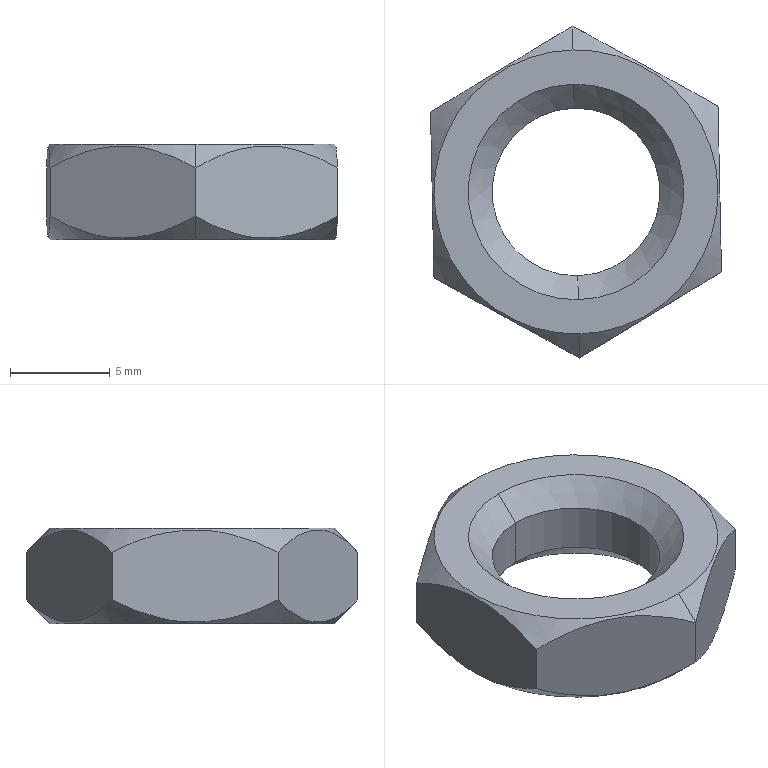Part | SolidWorks | features BaseBody 1 | 1 solid | 18 faces | box 14.572 x 16.624 x 4.802 mm | volume 539.911 mm3 | cone 8 | plane 8 | cylinder 2 | commonest cylinder face diameters 8.4 x2
STEP:
#1=CARTESIAN_POINT('',(341.861,193.205,-8.525));
#2=VERTEX_POINT('',#1);
#3=CARTESIAN_POINT('',(341.685,201.603,-8.525));
#4=VERTEX_POINT('',#3);
#5=CARTESIAN_POINT('',(341.773,197.404,-8.525));
#6=DIRECTION('',(-0.0001435,-0.000000521,1.));
#7=DIRECTION('',(0.02104,-0.9998,0.000002497));
#8=AXIS2_PLACEMENT_3D('',#5,#6,#7);
#9=CIRCLE('',#8,4.2);
#10=EDGE_CURVE('',#2,#4,#9,.T.);
#11=ORIENTED_EDGE('',*,*,#10,.T.);
#12=CARTESIAN_POINT('',(341.659,202.802,-9.725));
#13=VERTEX_POINT('',#12);
#14=CARTESIAN_POINT('',(341.672,202.203,-9.125));
#15=DIRECTION('',(-0.01477,0.707,-0.7071));
#16=VECTOR('',#15,1000.);
#17=LINE('',#14,#16);
#18=EDGE_CURVE('',#4,#13,#17,.T.);
#19=ORIENTED_EDGE('',*,*,#18,.T.);
#20=CARTESIAN_POINT('',(341.887,192.005,-9.725));
#21=VERTEX_POINT('',#20);
#22=CARTESIAN_POINT('',(341.773,197.404,-9.725));
#23=DIRECTION('',(-0.0001435,-0.000000521,1.));
#24=DIRECTION('',(-0.02104,0.9998,-0.000002497));
#25=AXIS2_PLACEMENT_3D('',#22,#23,#24);
#26=CIRCLE('',#25,5.4);
#27=EDGE_CURVE('',#21,#13,#26,.T.);
#28=ORIENTED_EDGE('',*,*,#27,.F.);
#29=CARTESIAN_POINT('',(341.874,192.605,-9.125));
#30=DIRECTION('',(0.01498,-0.7069,-0.7071));
#31=VECTOR('',#30,1000.);
#32=LINE('',#29,#31);
#33=EDGE_CURVE('',#2,#21,#32,.T.);
#34=ORIENTED_EDGE('',*,*,#33,.F.);
#35=EDGE_LOOP('',(#11,#19,#28,#34));
#36=FACE_OUTER_BOUND('',#35,.T.);
#37=CARTESIAN_POINT('',(341.773,197.404,-9.125));
#38=DIRECTION('',(0.0001435,0.000000521,-1.));
#39=DIRECTION('',(0.02104,-0.9998,0.000002497));
#40=AXIS2_PLACEMENT_3D('',#37,#38,#39);
#41=CONICAL_SURFACE('',#40,4.8,0.7854);
#42=ADVANCED_FACE('',(#36),#41,.F.);
#43=CARTESIAN_POINT('',(341.684,201.603,-6.125));
#44=VERTEX_POINT('',#43);
#45=CARTESIAN_POINT('',(341.861,193.205,-6.125));
#46=VERTEX_POINT('',#45);
#47=CARTESIAN_POINT('',(341.773,197.404,-6.125));
#48=DIRECTION('',(0.0001435,0.000000521,-1.));
#49=DIRECTION('',(0.02104,-0.9998,0.000002497));
#50=AXIS2_PLACEMENT_3D('',#47,#48,#49);
#51=CIRCLE('',#50,4.2);
#52=EDGE_CURVE('',#44,#46,#51,.T.);
#53=ORIENTED_EDGE('',*,*,#52,.F.);
#54=CARTESIAN_POINT('',(341.684,201.603,-3.125));
#55=DIRECTION('',(0.0001435,0.000000521,-1.));
#56=VECTOR('',#55,1000.);
#57=LINE('',#54,#56);
#58=EDGE_CURVE('',#44,#4,#57,.T.);
#59=ORIENTED_EDGE('',*,*,#58,.T.);
#60=ORIENTED_EDGE('',*,*,#10,.F.);
#61=CARTESIAN_POINT('',(341.86,193.205,-3.125));
#62=DIRECTION('',(0.0001435,0.000000521,-1.));
#63=VECTOR('',#62,1000.);
#64=LINE('',#61,#63);
#65=EDGE_CURVE('',#46,#2,#64,.T.);
#66=ORIENTED_EDGE('',*,*,#65,.F.);
#67=EDGE_LOOP('',(#53,#59,#60,#66));
#68=FACE_OUTER_BOUND('',#67,.T.);
#69=CARTESIAN_POINT('',(341.772,197.404,-3.125));
#70=DIRECTION('',(0.0001435,0.000000521,-1.));
#71=DIRECTION('',(0.02104,-0.9998,0.000002497));
#72=AXIS2_PLACEMENT_3D('',#69,#70,#71);
#73=CYLINDRICAL_SURFACE('',#72,4.2);
#74=ADVANCED_FACE('',(#68),#73,.F.);
#75=ORIENTED_EDGE('',*,*,#52,.T.);
#76=CARTESIAN_POINT('',(341.886,192.005,-4.925));
#77=VERTEX_POINT('',#76);
#78=CARTESIAN_POINT('',(341.873,192.605,-5.525));
#79=DIRECTION('',(0.01477,-0.707,0.7071));
#80=VECTOR('',#79,1000.);
#81=LINE('',#78,#80);
#82=EDGE_CURVE('',#46,#77,#81,.T.);
#83=ORIENTED_EDGE('',*,*,#82,.T.);
#84=CARTESIAN_POINT('',(341.659,202.802,-4.925));
#85=VERTEX_POINT('',#84);
#86=CARTESIAN_POINT('',(341.772,197.404,-4.925));
#87=DIRECTION('',(0.0001435,0.000000521,-1.));
#88=DIRECTION('',(0.02104,-0.9998,0.000002497));
#89=AXIS2_PLACEMENT_3D('',#86,#87,#88);
#90=CIRCLE('',#89,5.4);
#91=EDGE_CURVE('',#85,#77,#90,.T.);
#92=ORIENTED_EDGE('',*,*,#91,.F.);
#93=CARTESIAN_POINT('',(341.671,202.203,-5.525));
#94=DIRECTION('',(-0.01498,0.7069,0.7071));
#95=VECTOR('',#94,1000.);
#96=LINE('',#93,#95);
#97=EDGE_CURVE('',#44,#85,#96,.T.);
#98=ORIENTED_EDGE('',*,*,#97,.F.);
#99=EDGE_LOOP('',(#75,#83,#92,#98));
#100=FACE_OUTER_BOUND('',#99,.T.);
#101=CARTESIAN_POINT('',(341.772,197.404,-5.525));
#102=DIRECTION('',(-0.0001435,-0.000000521,1.));
#103=DIRECTION('',(-0.02104,0.9998,-0.000002497));
#104=AXIS2_PLACEMENT_3D('',#101,#102,#103);
#105=CONICAL_SURFACE('',#104,4.8,0.7854);
#106=ADVANCED_FACE('',(#100),#105,.F.);
#107=CARTESIAN_POINT('',(341.623,204.516,-4.925));
#108=VERTEX_POINT('',#107);
#109=CARTESIAN_POINT('',(341.922,190.291,-4.925));
#110=VERTEX_POINT('',#109);
#111=CARTESIAN_POINT('',(341.772,197.404,-4.925));
#112=DIRECTION('',(-0.0001435,-0.000000521,1.));
#113=DIRECTION('',(0.02104,-0.9998,0.000002497));
#114=AXIS2_PLACEMENT_3D('',#111,#112,#113);
#115=CIRCLE('',#114,7.114);
#116=EDGE_CURVE('',#108,#110,#115,.T.);
#117=ORIENTED_EDGE('',*,*,#116,.F.);
#118=CARTESIAN_POINT('',(341.598,205.716,-6.125));
#119=VERTEX_POINT('',#118);
#120=CARTESIAN_POINT('',(341.61,205.116,-5.525));
#121=DIRECTION('',(-0.01477,0.707,-0.7071));
#122=VECTOR('',#121,1000.);
#123=LINE('',#120,#122);
#124=EDGE_CURVE('',#108,#119,#123,.T.);
#125=ORIENTED_EDGE('',*,*,#124,.T.);
#126=CARTESIAN_POINT('',(334.487,201.408,-6.126));
#127=VERTEX_POINT('',#126);
#128=CARTESIAN_POINT('',(341.598,205.716,-6.125));
#129=CARTESIAN_POINT('',(341.463,205.634,-6.047));
#130=CARTESIAN_POINT('',(341.198,205.473,-5.899));
#131=CARTESIAN_POINT('',(340.818,205.243,-5.706));
#132=CARTESIAN_POINT('',(340.45,205.021,-5.539));
#133=CARTESIAN_POINT('',(340.092,204.803,-5.397));
#134=CARTESIAN_POINT('',(339.738,204.589,-5.277));
#135=CARTESIAN_POINT('',(339.391,204.379,-5.179));
#136=CARTESIAN_POINT('',(339.049,204.172,-5.104));
#137=CARTESIAN_POINT('',(338.711,203.967,-5.051));
#138=CARTESIAN_POINT('',(338.375,203.764,-5.019));
#139=CARTESIAN_POINT('',(338.04,203.561,-5.009));
#140=CARTESIAN_POINT('',(337.705,203.358,-5.019));
#141=CARTESIAN_POINT('',(337.369,203.154,-5.052));
#142=CARTESIAN_POINT('',(337.031,202.95,-5.105));
#143=CARTESIAN_POINT('',(336.69,202.743,-5.18));
#144=CARTESIAN_POINT('',(336.344,202.533,-5.278));
#145=CARTESIAN_POINT('',(335.992,202.32,-5.398));
#146=CARTESIAN_POINT('',(335.634,202.103,-5.54));
#147=CARTESIAN_POINT('',(335.267,201.881,-5.707));
#148=CARTESIAN_POINT('',(334.887,201.65,-5.899));
#149=CARTESIAN_POINT('',(334.622,201.49,-6.047));
#150=CARTESIAN_POINT('',(334.487,201.408,-6.126));
#151=B_SPLINE_CURVE_WITH_KNOTS('',3,(#128,#129,#130,#131,#132,#133,#134,#135,#136,#137,#138,#139,#140,#141,#142,#143,#144,#145,#146,#147,#148,#149,#150),.UNSPECIFIED.,.F.,.F.,(4,1,1,1,1,1,1,1,1,1,1,1,1,1,1,1,1,1,1,1,4),(0.,0.05,0.1,0.15,0.2,0.25,0.3,0.35,0.4,0.45,0.5,0.55,0.6,0.65,0.7,0.75,0.8,0.85,0.9,0.95,1.),.UNSPECIFIED.);
#152=EDGE_CURVE('',#119,#127,#151,.T.);
#153=ORIENTED_EDGE('',*,*,#152,.T.);
#154=CARTESIAN_POINT('',(334.662,193.096,-6.126));
#155=VERTEX_POINT('',#154);
#156=CARTESIAN_POINT('',(334.487,201.408,-6.126));
#157=CARTESIAN_POINT('',(334.5,200.759,-5.802));
#158=CARTESIAN_POINT('',(334.514,200.095,-5.526));
#159=CARTESIAN_POINT('',(334.536,199.063,-5.23));
#160=CARTESIAN_POINT('',(334.543,198.713,-5.151));
#161=CARTESIAN_POINT('',(334.558,197.998,-5.043));
#162=CARTESIAN_POINT('',(334.566,197.63,-5.013));
#163=CARTESIAN_POINT('',(334.589,196.542,-5.011));
#164=CARTESIAN_POINT('',(334.604,195.829,-5.121));
#165=CARTESIAN_POINT('',(334.634,194.422,-5.52));
#166=CARTESIAN_POINT('',(334.648,193.749,-5.8));
#167=CARTESIAN_POINT('',(334.662,193.096,-6.126));
#168=B_SPLINE_CURVE_WITH_KNOTS('',3,(#156,#157,#158,#159,#160,#161,#162,#163,#164,#165,#166,#167),.UNSPECIFIED.,.F.,.F.,(4,2,2,2,2,4),(0.,0.002147,0.00322,0.004294,0.006441,0.008588),.UNSPECIFIED.);
#169=EDGE_CURVE('',#127,#155,#168,.T.);
#170=ORIENTED_EDGE('',*,*,#169,.T.);
#171=CARTESIAN_POINT('',(341.947,189.092,-6.125));
#172=VERTEX_POINT('',#171);
#173=CARTESIAN_POINT('',(334.662,193.096,-6.126));
#174=CARTESIAN_POINT('',(334.8,193.02,-6.048));
#175=CARTESIAN_POINT('',(335.071,192.871,-5.899));
#176=CARTESIAN_POINT('',(335.461,192.657,-5.707));
#177=CARTESIAN_POINT('',(335.837,192.45,-5.54));
#178=CARTESIAN_POINT('',(336.204,192.248,-5.397));
#179=CARTESIAN_POINT('',(336.566,192.049,-5.277));
#180=CARTESIAN_POINT('',(336.922,191.853,-5.179));
#181=CARTESIAN_POINT('',(337.273,191.661,-5.104));
#182=CARTESIAN_POINT('',(337.619,191.471,-5.051));
#183=CARTESIAN_POINT('',(337.963,191.281,-5.019));
#184=CARTESIAN_POINT('',(338.306,191.093,-5.009));
#185=CARTESIAN_POINT('',(338.649,190.904,-5.019));
#186=CARTESIAN_POINT('',(338.994,190.715,-5.051));
#187=CARTESIAN_POINT('',(339.34,190.525,-5.105));
#188=CARTESIAN_POINT('',(339.69,190.332,-5.18));
#189=CARTESIAN_POINT('',(340.044,190.137,-5.277));
#190=CARTESIAN_POINT('',(340.405,189.939,-5.397));
#191=CARTESIAN_POINT('',(340.772,189.738,-5.539));
#192=CARTESIAN_POINT('',(341.148,189.531,-5.706));
#193=CARTESIAN_POINT('',(341.537,189.317,-5.898));
#194=CARTESIAN_POINT('',(341.809,189.168,-6.046));
#195=CARTESIAN_POINT('',(341.947,189.092,-6.125));
#196=B_SPLINE_CURVE_WITH_KNOTS('',3,(#173,#174,#175,#176,#177,#178,#179,#180,#181,#182,#183,#184,#185,#186,#187,#188,#189,#190,#191,#192,#193,#194,#195),.UNSPECIFIED.,.F.,.F.,(4,1,1,1,1,1,1,1,1,1,1,1,1,1,1,1,1,1,1,1,4),(0.,0.05,0.1,0.15,0.2,0.25,0.3,0.35,0.4,0.45,0.5,0.55,0.6,0.65,0.7,0.75,0.8,0.85,0.9,0.95,1.),.UNSPECIFIED.);
#197=EDGE_CURVE('',#155,#172,#196,.T.);
#198=ORIENTED_EDGE('',*,*,#197,.T.);
#199=CARTESIAN_POINT('',(341.935,189.691,-5.525));
#200=DIRECTION('',(0.01498,-0.7069,-0.7071));
#201=VECTOR('',#200,1000.);
#202=LINE('',#199,#201);
#203=EDGE_CURVE('',#110,#172,#202,.T.);
#204=ORIENTED_EDGE('',*,*,#203,.F.);
#205=EDGE_LOOP('',(#117,#125,#153,#170,#198,#204));
#206=FACE_OUTER_BOUND('',#205,.T.);
#207=CARTESIAN_POINT('',(341.772,197.404,-5.525));
#208=DIRECTION('',(0.0001435,0.000000521,-1.));
#209=DIRECTION('',(0.02104,-0.9998,0.000002497));
#210=AXIS2_PLACEMENT_3D('',#207,#208,#209);
#211=CONICAL_SURFACE('',#210,7.714,0.7854);
#212=ADVANCED_FACE('',(#206),#211,.T.);
#213=CARTESIAN_POINT('',(341.923,190.291,-9.725));
#214=VERTEX_POINT('',#213);
#215=CARTESIAN_POINT('',(341.623,204.516,-9.725));
#216=VERTEX_POINT('',#215);
#217=CARTESIAN_POINT('',(341.773,197.404,-9.725));
#218=DIRECTION('',(0.0001435,0.000000521,-1.));
#219=DIRECTION('',(-0.02104,0.9998,-0.000002497));
#220=AXIS2_PLACEMENT_3D('',#217,#218,#219);
#221=CIRCLE('',#220,7.114);
#222=EDGE_CURVE('',#214,#216,#221,.T.);
#223=ORIENTED_EDGE('',*,*,#222,.F.);
#224=CARTESIAN_POINT('',(341.948,189.092,-8.525));
#225=VERTEX_POINT('',#224);
#226=CARTESIAN_POINT('',(341.935,189.691,-9.125));
#227=DIRECTION('',(0.01477,-0.707,0.7071));
#228=VECTOR('',#227,1000.);
#229=LINE('',#226,#228);
#230=EDGE_CURVE('',#214,#225,#229,.T.);
#231=ORIENTED_EDGE('',*,*,#230,.T.);
#232=CARTESIAN_POINT('',(334.662,193.096,-8.526));
#233=VERTEX_POINT('',#232);
#234=CARTESIAN_POINT('',(341.948,189.092,-8.525));
#235=CARTESIAN_POINT('',(341.809,189.168,-8.604));
#236=CARTESIAN_POINT('',(341.538,189.317,-8.752));
#237=CARTESIAN_POINT('',(341.149,189.531,-8.945));
#238=CARTESIAN_POINT('',(340.772,189.738,-9.112));
#239=CARTESIAN_POINT('',(340.405,189.94,-9.255));
#240=CARTESIAN_POINT('',(340.043,190.138,-9.375));
#241=CARTESIAN_POINT('',(339.687,190.334,-9.472));
#242=CARTESIAN_POINT('',(339.337,190.527,-9.548));
#243=CARTESIAN_POINT('',(338.99,190.717,-9.601));
#244=CARTESIAN_POINT('',(338.646,190.906,-9.633));
#245=CARTESIAN_POINT('',(338.303,191.095,-9.643));
#246=CARTESIAN_POINT('',(337.96,191.283,-9.633));
#247=CARTESIAN_POINT('',(337.616,191.473,-9.601));
#248=CARTESIAN_POINT('',(337.269,191.663,-9.547));
#249=CARTESIAN_POINT('',(336.92,191.855,-9.472));
#250=CARTESIAN_POINT('',(336.565,192.05,-9.375));
#251=CARTESIAN_POINT('',(336.204,192.248,-9.255));
#252=CARTESIAN_POINT('',(335.838,192.45,-9.113));
#253=CARTESIAN_POINT('',(335.461,192.657,-8.946));
#254=CARTESIAN_POINT('',(335.072,192.871,-8.754));
#255=CARTESIAN_POINT('',(334.8,193.02,-8.605));
#256=CARTESIAN_POINT('',(334.662,193.096,-8.526));
#257=B_SPLINE_CURVE_WITH_KNOTS('',3,(#234,#235,#236,#237,#238,#239,#240,#241,#242,#243,#244,#245,#246,#247,#248,#249,#250,#251,#252,#253,#254,#255,#256),.UNSPECIFIED.,.F.,.F.,(4,1,1,1,1,1,1,1,1,1,1,1,1,1,1,1,1,1,1,1,4),(0.,0.05,0.1,0.15,0.2,0.25,0.3,0.35,0.4,0.45,0.5,0.55,0.6,0.65,0.7,0.75,0.8,0.85,0.9,0.95,1.),.UNSPECIFIED.);
#258=EDGE_CURVE('',#225,#233,#257,.T.);
#259=ORIENTED_EDGE('',*,*,#258,.T.);
#260=CARTESIAN_POINT('',(334.487,201.408,-8.526));
#261=VERTEX_POINT('',#260);
#262=CARTESIAN_POINT('',(334.662,193.096,-8.526));
#263=CARTESIAN_POINT('',(334.648,193.746,-8.851));
#264=CARTESIAN_POINT('',(334.634,194.41,-9.127));
#265=CARTESIAN_POINT('',(334.613,195.441,-9.423));
#266=CARTESIAN_POINT('',(334.605,195.791,-9.502));
#267=CARTESIAN_POINT('',(334.59,196.506,-9.61));
#268=CARTESIAN_POINT('',(334.583,196.874,-9.64));
#269=CARTESIAN_POINT('',(334.56,197.962,-9.642));
#270=CARTESIAN_POINT('',(334.545,198.676,-9.532));
#271=CARTESIAN_POINT('',(334.515,200.082,-9.133));
#272=CARTESIAN_POINT('',(334.501,200.755,-8.853));
#273=CARTESIAN_POINT('',(334.487,201.408,-8.526));
#274=B_SPLINE_CURVE_WITH_KNOTS('',3,(#262,#263,#264,#265,#266,#267,#268,#269,#270,#271,#272,#273),.UNSPECIFIED.,.F.,.F.,(4,2,2,2,2,4),(0.,0.002147,0.00322,0.004294,0.006441,0.008588),.UNSPECIFIED.);
#275=EDGE_CURVE('',#233,#261,#274,.T.);
#276=ORIENTED_EDGE('',*,*,#275,.T.);
#277=CARTESIAN_POINT('',(341.598,205.716,-8.525));
#278=VERTEX_POINT('',#277);
#279=CARTESIAN_POINT('',(334.487,201.408,-8.526));
#280=CARTESIAN_POINT('',(334.622,201.49,-8.605));
#281=CARTESIAN_POINT('',(334.887,201.65,-8.753));
#282=CARTESIAN_POINT('',(335.267,201.88,-8.946));
#283=CARTESIAN_POINT('',(335.634,202.103,-9.113));
#284=CARTESIAN_POINT('',(335.993,202.32,-9.255));
#285=CARTESIAN_POINT('',(336.346,202.534,-9.375));
#286=CARTESIAN_POINT('',(336.694,202.745,-9.473));
#287=CARTESIAN_POINT('',(337.036,202.952,-9.548));
#288=CARTESIAN_POINT('',(337.374,203.157,-9.601));
#289=CARTESIAN_POINT('',(337.71,203.36,-9.633));
#290=CARTESIAN_POINT('',(338.044,203.563,-9.643));
#291=CARTESIAN_POINT('',(338.379,203.766,-9.633));
#292=CARTESIAN_POINT('',(338.715,203.969,-9.6));
#293=CARTESIAN_POINT('',(339.053,204.174,-9.547));
#294=CARTESIAN_POINT('',(339.395,204.381,-9.472));
#295=CARTESIAN_POINT('',(339.741,204.591,-9.374));
#296=CARTESIAN_POINT('',(340.093,204.804,-9.254));
#297=CARTESIAN_POINT('',(340.451,205.02,-9.112));
#298=CARTESIAN_POINT('',(340.818,205.243,-8.945));
#299=CARTESIAN_POINT('',(341.198,205.473,-8.753));
#300=CARTESIAN_POINT('',(341.463,205.634,-8.604));
#301=CARTESIAN_POINT('',(341.598,205.716,-8.525));
#302=B_SPLINE_CURVE_WITH_KNOTS('',3,(#279,#280,#281,#282,#283,#284,#285,#286,#287,#288,#289,#290,#291,#292,#293,#294,#295,#296,#297,#298,#299,#300,#301),.UNSPECIFIED.,.F.,.F.,(4,1,1,1,1,1,1,1,1,1,1,1,1,1,1,1,1,1,1,1,4),(0.,0.05,0.1,0.15,0.2,0.25,0.3,0.35,0.4,0.45,0.5,0.55,0.6,0.65,0.7,0.75,0.8,0.85,0.9,0.95,1.),.UNSPECIFIED.);
#303=EDGE_CURVE('',#261,#278,#302,.T.);
#304=ORIENTED_EDGE('',*,*,#303,.T.);
#305=CARTESIAN_POINT('',(341.611,205.116,-9.125));
#306=DIRECTION('',(-0.01498,0.7069,0.7071));
#307=VECTOR('',#306,1000.);
#308=LINE('',#305,#307);
#309=EDGE_CURVE('',#216,#278,#308,.T.);
#310=ORIENTED_EDGE('',*,*,#309,.F.);
#311=EDGE_LOOP('',(#223,#231,#259,#276,#304,#310));
#312=FACE_OUTER_BOUND('',#311,.T.);
#313=CARTESIAN_POINT('',(341.773,197.404,-9.125));
#314=DIRECTION('',(-0.0001435,-0.000000521,1.));
#315=DIRECTION('',(-0.02104,0.9998,-0.000002497));
#316=AXIS2_PLACEMENT_3D('',#313,#314,#315);
#317=CONICAL_SURFACE('',#316,7.714,0.7854);
#318=ADVANCED_FACE('',(#312),#317,.T.);
#319=CARTESIAN_POINT('',(348.884,201.711,-8.524));
#320=VERTEX_POINT('',#319);
#321=CARTESIAN_POINT('',(348.883,201.711,-6.124));
#322=VERTEX_POINT('',#321);
#323=CARTESIAN_POINT('',(348.884,201.711,-8.524));
#324=DIRECTION('',(-0.0001435,-0.000000521,1.));
#325=VECTOR('',#324,1000.);
#326=LINE('',#323,#325);
#327=EDGE_CURVE('',#320,#322,#326,.T.);
#328=ORIENTED_EDGE('',*,*,#327,.T.);
#329=CARTESIAN_POINT('',(349.058,193.399,-6.124));
#330=VERTEX_POINT('',#329);
#331=CARTESIAN_POINT('',(349.058,193.399,-6.124));
#332=CARTESIAN_POINT('',(349.045,194.048,-5.8));
#333=CARTESIAN_POINT('',(349.031,194.713,-5.523));
#334=CARTESIAN_POINT('',(349.009,195.744,-5.228));
#335=CARTESIAN_POINT('',(349.002,196.094,-5.149));
#336=CARTESIAN_POINT('',(348.986,196.809,-5.041));
#337=CARTESIAN_POINT('',(348.979,197.177,-5.011));
#338=CARTESIAN_POINT('',(348.956,198.265,-5.009));
#339=CARTESIAN_POINT('',(348.941,198.979,-5.119));
#340=CARTESIAN_POINT('',(348.911,200.385,-5.518));
#341=CARTESIAN_POINT('',(348.897,201.058,-5.798));
#342=CARTESIAN_POINT('',(348.883,201.711,-6.124));
#343=B_SPLINE_CURVE_WITH_KNOTS('',3,(#331,#332,#333,#334,#335,#336,#337,#338,#339,#340,#341,#342),.UNSPECIFIED.,.F.,.F.,(4,2,2,2,2,4),(0.,0.002147,0.00322,0.004294,0.006441,0.008588),.UNSPECIFIED.);
#344=EDGE_CURVE('',#330,#322,#343,.T.);
#345=ORIENTED_EDGE('',*,*,#344,.F.);
#346=CARTESIAN_POINT('',(349.059,193.399,-8.524));
#347=VERTEX_POINT('',#346);
#348=CARTESIAN_POINT('',(349.059,193.399,-8.524));
#349=DIRECTION('',(-0.0001435,-0.000000521,1.));
#350=VECTOR('',#349,1000.);
#351=LINE('',#348,#350);
#352=EDGE_CURVE('',#347,#330,#351,.T.);
#353=ORIENTED_EDGE('',*,*,#352,.F.);
#354=CARTESIAN_POINT('',(348.884,201.711,-8.524));
#355=CARTESIAN_POINT('',(348.898,201.062,-8.849));
#356=CARTESIAN_POINT('',(348.912,200.398,-9.125));
#357=CARTESIAN_POINT('',(348.933,199.366,-9.421));
#358=CARTESIAN_POINT('',(348.941,199.016,-9.5));
#359=CARTESIAN_POINT('',(348.956,198.301,-9.608));
#360=CARTESIAN_POINT('',(348.963,197.933,-9.637));
#361=CARTESIAN_POINT('',(348.986,196.845,-9.64));
#362=CARTESIAN_POINT('',(349.001,196.132,-9.53));
#363=CARTESIAN_POINT('',(349.031,194.725,-9.131));
#364=CARTESIAN_POINT('',(349.045,194.052,-8.851));
#365=CARTESIAN_POINT('',(349.059,193.399,-8.524));
#366=B_SPLINE_CURVE_WITH_KNOTS('',3,(#354,#355,#356,#357,#358,#359,#360,#361,#362,#363,#364,#365),.UNSPECIFIED.,.F.,.F.,(4,2,2,2,2,4),(0.,0.002147,0.00322,0.004294,0.006441,0.008588),.UNSPECIFIED.);
#367=EDGE_CURVE('',#320,#347,#366,.T.);
#368=ORIENTED_EDGE('',*,*,#367,.F.);
#369=EDGE_LOOP('',(#328,#345,#353,#368));
#370=FACE_OUTER_BOUND('',#369,.T.);
#371=CARTESIAN_POINT('',(349.059,193.399,-9.724));
#372=DIRECTION('',(-0.9998,-0.02104,-0.0001435));
#373=DIRECTION('',(-0.02104,0.9998,0.));
#374=AXIS2_PLACEMENT_3D('',#371,#372,#373);
#375=PLANE('',#374);
#376=ADVANCED_FACE('',(#370),#375,.F.);
#377=ORIENTED_EDGE('',*,*,#352,.T.);
#378=CARTESIAN_POINT('',(341.947,189.092,-6.125));
#379=CARTESIAN_POINT('',(342.082,189.173,-6.046));
#380=CARTESIAN_POINT('',(342.347,189.334,-5.898));
#381=CARTESIAN_POINT('',(342.727,189.564,-5.706));
#382=CARTESIAN_POINT('',(343.095,189.787,-5.539));
#383=CARTESIAN_POINT('',(343.453,190.004,-5.396));
#384=CARTESIAN_POINT('',(343.806,190.218,-5.276));
#385=CARTESIAN_POINT('',(344.154,190.428,-5.178));
#386=CARTESIAN_POINT('',(344.496,190.635,-5.103));
#387=CARTESIAN_POINT('',(344.834,190.84,-5.05));
#388=CARTESIAN_POINT('',(345.17,191.044,-5.018));
#389=CARTESIAN_POINT('',(345.504,191.246,-5.008));
#390=CARTESIAN_POINT('',(345.839,191.449,-5.018));
#391=CARTESIAN_POINT('',(346.176,191.653,-5.05));
#392=CARTESIAN_POINT('',(346.513,191.858,-5.104));
#393=CARTESIAN_POINT('',(346.855,192.064,-5.179));
#394=CARTESIAN_POINT('',(347.201,192.274,-5.276));
#395=CARTESIAN_POINT('',(347.553,192.487,-5.396));
#396=CARTESIAN_POINT('',(347.911,192.704,-5.538));
#397=CARTESIAN_POINT('',(348.278,192.926,-5.705));
#398=CARTESIAN_POINT('',(348.658,193.157,-5.897));
#399=CARTESIAN_POINT('',(348.923,193.317,-6.045));
#400=CARTESIAN_POINT('',(349.058,193.399,-6.124));
#401=B_SPLINE_CURVE_WITH_KNOTS('',3,(#378,#379,#380,#381,#382,#383,#384,#385,#386,#387,#388,#389,#390,#391,#392,#393,#394,#395,#396,#397,#398,#399,#400),.UNSPECIFIED.,.F.,.F.,(4,1,1,1,1,1,1,1,1,1,1,1,1,1,1,1,1,1,1,1,4),(0.,0.05,0.1,0.15,0.2,0.25,0.3,0.35,0.4,0.45,0.5,0.55,0.6,0.65,0.7,0.75,0.8,0.85,0.9,0.95,1.),.UNSPECIFIED.);
#402=EDGE_CURVE('',#172,#330,#401,.T.);
#403=ORIENTED_EDGE('',*,*,#402,.F.);
#404=CARTESIAN_POINT('',(341.948,189.092,-8.525));
#405=DIRECTION('',(-0.0001435,-0.000000521,1.));
#406=VECTOR('',#405,1000.);
#407=LINE('',#404,#406);
#408=EDGE_CURVE('',#225,#172,#407,.T.);
#409=ORIENTED_EDGE('',*,*,#408,.F.);
#410=CARTESIAN_POINT('',(349.059,193.399,-8.524));
#411=CARTESIAN_POINT('',(348.924,193.317,-8.603));
#412=CARTESIAN_POINT('',(348.659,193.157,-8.751));
#413=CARTESIAN_POINT('',(348.279,192.927,-8.944));
#414=CARTESIAN_POINT('',(347.912,192.704,-9.111));
#415=CARTESIAN_POINT('',(347.553,192.487,-9.254));
#416=CARTESIAN_POINT('',(347.2,192.273,-9.374));
#417=CARTESIAN_POINT('',(346.852,192.062,-9.471));
#418=CARTESIAN_POINT('',(346.51,191.855,-9.547));
#419=CARTESIAN_POINT('',(346.172,191.65,-9.6));
#420=CARTESIAN_POINT('',(345.836,191.447,-9.632));
#421=CARTESIAN_POINT('',(345.502,191.244,-9.642));
#422=CARTESIAN_POINT('',(345.167,191.041,-9.632));
#423=CARTESIAN_POINT('',(344.831,190.838,-9.6));
#424=CARTESIAN_POINT('',(344.493,190.633,-9.546));
#425=CARTESIAN_POINT('',(344.151,190.426,-9.471));
#426=CARTESIAN_POINT('',(343.805,190.217,-9.374));
#427=CARTESIAN_POINT('',(343.453,190.003,-9.254));
#428=CARTESIAN_POINT('',(343.095,189.787,-9.112));
#429=CARTESIAN_POINT('',(342.728,189.564,-8.945));
#430=CARTESIAN_POINT('',(342.348,189.334,-8.752));
#431=CARTESIAN_POINT('',(342.083,189.173,-8.604));
#432=CARTESIAN_POINT('',(341.948,189.092,-8.525));
#433=B_SPLINE_CURVE_WITH_KNOTS('',3,(#410,#411,#412,#413,#414,#415,#416,#417,#418,#419,#420,#421,#422,#423,#424,#425,#426,#427,#428,#429,#430,#431,#432),.UNSPECIFIED.,.F.,.F.,(4,1,1,1,1,1,1,1,1,1,1,1,1,1,1,1,1,1,1,1,4),(0.,0.05,0.1,0.15,0.2,0.25,0.3,0.35,0.4,0.45,0.5,0.55,0.6,0.65,0.7,0.75,0.8,0.85,0.9,0.95,1.),.UNSPECIFIED.);
#434=EDGE_CURVE('',#347,#225,#433,.T.);
#435=ORIENTED_EDGE('',*,*,#434,.F.);
#436=EDGE_LOOP('',(#377,#403,#409,#435));
#437=FACE_OUTER_BOUND('',#436,.T.);
#438=CARTESIAN_POINT('',(341.948,189.092,-9.725));
#439=DIRECTION('',(-0.5181,0.8553,-0.00007389));
#440=DIRECTION('',(-0.0001426,0.,1.));
#441=AXIS2_PLACEMENT_3D('',#438,#439,#440);
#442=PLANE('',#441);
#443=ADVANCED_FACE('',(#437),#442,.F.);
#444=ORIENTED_EDGE('',*,*,#408,.T.);
#445=ORIENTED_EDGE('',*,*,#197,.F.);
#446=CARTESIAN_POINT('',(334.662,193.096,-8.526));
#447=DIRECTION('',(-0.0001435,-0.000000521,1.));
#448=VECTOR('',#447,1000.);
#449=LINE('',#446,#448);
#450=EDGE_CURVE('',#233,#155,#449,.T.);
#451=ORIENTED_EDGE('',*,*,#450,.F.);
#452=ORIENTED_EDGE('',*,*,#258,.F.);
#453=EDGE_LOOP('',(#444,#445,#451,#452));
#454=FACE_OUTER_BOUND('',#453,.T.);
#455=CARTESIAN_POINT('',(334.662,193.096,-9.726));
#456=DIRECTION('',(0.4817,0.8764,0.00006956));
#457=DIRECTION('',(0.0001444,0.,-1.));
#458=AXIS2_PLACEMENT_3D('',#455,#456,#457);
#459=PLANE('',#458);
#460=ADVANCED_FACE('',(#454),#459,.F.);
#461=ORIENTED_EDGE('',*,*,#450,.T.);
#462=ORIENTED_EDGE('',*,*,#169,.F.);
#463=CARTESIAN_POINT('',(334.487,201.408,-8.526));
#464=DIRECTION('',(-0.0001435,-0.000000521,1.));
#465=VECTOR('',#464,1000.);
#466=LINE('',#463,#465);
#467=EDGE_CURVE('',#261,#127,#466,.T.);
#468=ORIENTED_EDGE('',*,*,#467,.F.);
#469=ORIENTED_EDGE('',*,*,#275,.F.);
#470=EDGE_LOOP('',(#461,#462,#468,#469));
#471=FACE_OUTER_BOUND('',#470,.T.);
#472=CARTESIAN_POINT('',(334.487,201.408,-9.726));
#473=DIRECTION('',(0.9998,0.02104,0.0001435));
#474=DIRECTION('',(0.,0.006819,-1.));
#475=AXIS2_PLACEMENT_3D('',#472,#473,#474);
#476=PLANE('',#475);
#477=ADVANCED_FACE('',(#471),#476,.F.);
#478=ORIENTED_EDGE('',*,*,#467,.T.);
#479=ORIENTED_EDGE('',*,*,#152,.F.);
#480=CARTESIAN_POINT('',(341.598,205.716,-8.525));
#481=DIRECTION('',(-0.0001435,-0.000000521,1.));
#482=VECTOR('',#481,1000.);
#483=LINE('',#480,#482);
#484=EDGE_CURVE('',#278,#119,#483,.T.);
#485=ORIENTED_EDGE('',*,*,#484,.F.);
#486=ORIENTED_EDGE('',*,*,#303,.F.);
#487=EDGE_LOOP('',(#478,#479,#485,#486));
#488=FACE_OUTER_BOUND('',#487,.T.);
#489=CARTESIAN_POINT('',(341.598,205.716,-9.725));
#490=DIRECTION('',(0.5181,-0.8553,0.00007389));
#491=DIRECTION('',(0.,-0.00008639,-1.));
#492=AXIS2_PLACEMENT_3D('',#489,#490,#491);
#493=PLANE('',#492);
#494=ADVANCED_FACE('',(#488),#493,.F.);
#495=ORIENTED_EDGE('',*,*,#230,.F.);
#496=CARTESIAN_POINT('',(341.773,197.404,-9.725));
#497=DIRECTION('',(0.0001435,0.000000521,-1.));
#498=DIRECTION('',(-0.02104,0.9998,-0.000002497));
#499=AXIS2_PLACEMENT_3D('',#496,#497,#498);
#500=CIRCLE('',#499,7.114);
#501=EDGE_CURVE('',#216,#214,#500,.T.);
#502=ORIENTED_EDGE('',*,*,#501,.F.);
#503=ORIENTED_EDGE('',*,*,#309,.T.);
#504=CARTESIAN_POINT('',(341.598,205.716,-8.525));
#505=CARTESIAN_POINT('',(341.736,205.64,-8.604));
#506=CARTESIAN_POINT('',(342.008,205.49,-8.752));
#507=CARTESIAN_POINT('',(342.397,205.276,-8.945));
#508=CARTESIAN_POINT('',(342.774,205.069,-9.112));
#509=CARTESIAN_POINT('',(343.141,204.868,-9.254));
#510=CARTESIAN_POINT('',(343.503,204.669,-9.374));
#511=CARTESIAN_POINT('',(343.859,204.473,-9.472));
#512=CARTESIAN_POINT('',(344.209,204.28,-9.547));
#513=CARTESIAN_POINT('',(344.556,204.09,-9.6));
#514=CARTESIAN_POINT('',(344.9,203.901,-9.632));
#515=CARTESIAN_POINT('',(345.243,203.712,-9.642));
#516=CARTESIAN_POINT('',(345.586,203.524,-9.632));
#517=CARTESIAN_POINT('',(345.93,203.334,-9.599));
#518=CARTESIAN_POINT('',(346.277,203.144,-9.546));
#519=CARTESIAN_POINT('',(346.626,202.952,-9.471));
#520=CARTESIAN_POINT('',(346.981,202.757,-9.373));
#521=CARTESIAN_POINT('',(347.342,202.559,-9.253));
#522=CARTESIAN_POINT('',(347.708,202.357,-9.111));
#523=CARTESIAN_POINT('',(348.085,202.15,-8.944));
#524=CARTESIAN_POINT('',(348.474,201.936,-8.752));
#525=CARTESIAN_POINT('',(348.745,201.787,-8.603));
#526=CARTESIAN_POINT('',(348.884,201.711,-8.524));
#527=B_SPLINE_CURVE_WITH_KNOTS('',3,(#504,#505,#506,#507,#508,#509,#510,#511,#512,#513,#514,#515,#516,#517,#518,#519,#520,#521,#522,#523,#524,#525,#526),.UNSPECIFIED.,.F.,.F.,(4,1,1,1,1,1,1,1,1,1,1,1,1,1,1,1,1,1,1,1,4),(0.,0.05,0.1,0.15,0.2,0.25,0.3,0.35,0.4,0.45,0.5,0.55,0.6,0.65,0.7,0.75,0.8,0.85,0.9,0.95,1.),.UNSPECIFIED.);
#528=EDGE_CURVE('',#278,#320,#527,.T.);
#529=ORIENTED_EDGE('',*,*,#528,.T.);
#530=ORIENTED_EDGE('',*,*,#367,.T.);
#531=ORIENTED_EDGE('',*,*,#434,.T.);
#532=EDGE_LOOP('',(#495,#502,#503,#529,#530,#531));
#533=FACE_OUTER_BOUND('',#532,.T.);
#534=CARTESIAN_POINT('',(341.773,197.404,-9.125));
#535=DIRECTION('',(-0.0001435,-0.000000521,1.));
#536=DIRECTION('',(-0.02104,0.9998,-0.000002497));
#537=AXIS2_PLACEMENT_3D('',#534,#535,#536);
#538=CONICAL_SURFACE('',#537,7.714,0.7854);
#539=ADVANCED_FACE('',(#533),#538,.T.);
#540=ORIENTED_EDGE('',*,*,#484,.T.);
#541=CARTESIAN_POINT('',(348.883,201.711,-6.124));
#542=CARTESIAN_POINT('',(348.745,201.787,-6.046));
#543=CARTESIAN_POINT('',(348.474,201.936,-5.897));
#544=CARTESIAN_POINT('',(348.084,202.15,-5.705));
#545=CARTESIAN_POINT('',(347.708,202.357,-5.538));
#546=CARTESIAN_POINT('',(347.341,202.559,-5.396));
#547=CARTESIAN_POINT('',(346.979,202.758,-5.276));
#548=CARTESIAN_POINT('',(346.622,202.954,-5.178));
#549=CARTESIAN_POINT('',(346.272,203.146,-5.103));
#550=CARTESIAN_POINT('',(345.926,203.337,-5.05));
#551=CARTESIAN_POINT('',(345.582,203.526,-5.018));
#552=CARTESIAN_POINT('',(345.239,203.714,-5.008));
#553=CARTESIAN_POINT('',(344.896,203.903,-5.018));
#554=CARTESIAN_POINT('',(344.551,204.092,-5.051));
#555=CARTESIAN_POINT('',(344.205,204.282,-5.104));
#556=CARTESIAN_POINT('',(343.855,204.475,-5.179));
#557=CARTESIAN_POINT('',(343.5,204.67,-5.277));
#558=CARTESIAN_POINT('',(343.14,204.868,-5.397));
#559=CARTESIAN_POINT('',(342.773,205.069,-5.539));
#560=CARTESIAN_POINT('',(342.397,205.276,-5.706));
#561=CARTESIAN_POINT('',(342.008,205.49,-5.898));
#562=CARTESIAN_POINT('',(341.736,205.639,-6.046));
#563=CARTESIAN_POINT('',(341.598,205.716,-6.125));
#564=B_SPLINE_CURVE_WITH_KNOTS('',3,(#541,#542,#543,#544,#545,#546,#547,#548,#549,#550,#551,#552,#553,#554,#555,#556,#557,#558,#559,#560,#561,#562,#563),.UNSPECIFIED.,.F.,.F.,(4,1,1,1,1,1,1,1,1,1,1,1,1,1,1,1,1,1,1,1,4),(0.,0.05,0.1,0.15,0.2,0.25,0.3,0.35,0.4,0.45,0.5,0.55,0.6,0.65,0.7,0.75,0.8,0.85,0.9,0.95,1.),.UNSPECIFIED.);
#565=EDGE_CURVE('',#322,#119,#564,.T.);
#566=ORIENTED_EDGE('',*,*,#565,.F.);
#567=ORIENTED_EDGE('',*,*,#327,.F.);
#568=ORIENTED_EDGE('',*,*,#528,.F.);
#569=EDGE_LOOP('',(#540,#566,#567,#568));
#570=FACE_OUTER_BOUND('',#569,.T.);
#571=CARTESIAN_POINT('',(348.884,201.711,-9.724));
#572=DIRECTION('',(-0.4817,-0.8764,-0.00006956));
#573=DIRECTION('',(-0.8764,0.4817,0.));
#574=AXIS2_PLACEMENT_3D('',#571,#572,#573);
#575=PLANE('',#574);
#576=ADVANCED_FACE('',(#570),#575,.F.);
#577=ORIENTED_EDGE('',*,*,#124,.F.);
#578=CARTESIAN_POINT('',(341.772,197.404,-4.925));
#579=DIRECTION('',(-0.0001435,-0.000000521,1.));
#580=DIRECTION('',(0.02104,-0.9998,0.000002497));
#581=AXIS2_PLACEMENT_3D('',#578,#579,#580);
#582=CIRCLE('',#581,7.114);
#583=EDGE_CURVE('',#110,#108,#582,.T.);
#584=ORIENTED_EDGE('',*,*,#583,.F.);
#585=ORIENTED_EDGE('',*,*,#203,.T.);
#586=ORIENTED_EDGE('',*,*,#402,.T.);
#587=ORIENTED_EDGE('',*,*,#344,.T.);
#588=ORIENTED_EDGE('',*,*,#565,.T.);
#589=EDGE_LOOP('',(#577,#584,#585,#586,#587,#588));
#590=FACE_OUTER_BOUND('',#589,.T.);
#591=CARTESIAN_POINT('',(341.772,197.404,-5.525));
#592=DIRECTION('',(0.0001435,0.000000521,-1.));
#593=DIRECTION('',(0.02104,-0.9998,0.000002497));
#594=AXIS2_PLACEMENT_3D('',#591,#592,#593);
#595=CONICAL_SURFACE('',#594,7.714,0.7854);
#596=ADVANCED_FACE('',(#590),#595,.T.);
#597=ORIENTED_EDGE('',*,*,#91,.T.);
#598=CARTESIAN_POINT('',(341.772,197.404,-4.925));
#599=DIRECTION('',(0.0001435,0.000000521,-1.));
#600=DIRECTION('',(0.02104,-0.9998,0.000002497));
#601=AXIS2_PLACEMENT_3D('',#598,#599,#600);
#602=CIRCLE('',#601,5.4);
#603=EDGE_CURVE('',#77,#85,#602,.T.);
#604=ORIENTED_EDGE('',*,*,#603,.T.);
#605=EDGE_LOOP('',(#597,#604));
#606=FACE_BOUND('',#605,.T.);
#607=ORIENTED_EDGE('',*,*,#583,.T.);
#608=ORIENTED_EDGE('',*,*,#116,.T.);
#609=EDGE_LOOP('',(#607,#608));
#610=FACE_OUTER_BOUND('',#609,.T.);
#611=CARTESIAN_POINT('',(341.16,226.497,-4.926));
#612=DIRECTION('',(0.0001435,0.000000521,-1.));
#613=DIRECTION('',(0.,-1.,-0.000000521));
#614=AXIS2_PLACEMENT_3D('',#611,#612,#613);
#615=PLANE('',#614);
#616=ADVANCED_FACE('',(#606,#610),#615,.F.);
#617=ORIENTED_EDGE('',*,*,#82,.F.);
#618=CARTESIAN_POINT('',(341.773,197.404,-6.125));
#619=DIRECTION('',(0.0001435,0.000000521,-1.));
#620=DIRECTION('',(0.02104,-0.9998,0.000002497));
#621=AXIS2_PLACEMENT_3D('',#618,#619,#620);
#622=CIRCLE('',#621,4.2);
#623=EDGE_CURVE('',#46,#44,#622,.T.);
#624=ORIENTED_EDGE('',*,*,#623,.T.);
#625=ORIENTED_EDGE('',*,*,#97,.T.);
#626=ORIENTED_EDGE('',*,*,#603,.F.);
#627=EDGE_LOOP('',(#617,#624,#625,#626));
#628=FACE_OUTER_BOUND('',#627,.T.);
#629=CARTESIAN_POINT('',(341.772,197.404,-5.525));
#630=DIRECTION('',(-0.0001435,-0.000000521,1.));
#631=DIRECTION('',(-0.02104,0.9998,-0.000002497));
#632=AXIS2_PLACEMENT_3D('',#629,#630,#631);
#633=CONICAL_SURFACE('',#632,4.8,0.7854);
#634=ADVANCED_FACE('',(#628),#633,.F.);
#635=ORIENTED_EDGE('',*,*,#58,.F.);
#636=ORIENTED_EDGE('',*,*,#623,.F.);
#637=ORIENTED_EDGE('',*,*,#65,.T.);
#638=CARTESIAN_POINT('',(341.773,197.404,-8.525));
#639=DIRECTION('',(-0.0001435,-0.000000521,1.));
#640=DIRECTION('',(0.02104,-0.9998,0.000002497));
#641=AXIS2_PLACEMENT_3D('',#638,#639,#640);
#642=CIRCLE('',#641,4.2);
#643=EDGE_CURVE('',#4,#2,#642,.T.);
#644=ORIENTED_EDGE('',*,*,#643,.F.);
#645=EDGE_LOOP('',(#635,#636,#637,#644));
#646=FACE_OUTER_BOUND('',#645,.T.);
#647=CARTESIAN_POINT('',(341.772,197.404,-3.125));
#648=DIRECTION('',(0.0001435,0.000000521,-1.));
#649=DIRECTION('',(0.02104,-0.9998,0.000002497));
#650=AXIS2_PLACEMENT_3D('',#647,#648,#649);
#651=CYLINDRICAL_SURFACE('',#650,4.2);
#652=ADVANCED_FACE('',(#646),#651,.F.);
#653=ORIENTED_EDGE('',*,*,#18,.F.);
#654=ORIENTED_EDGE('',*,*,#643,.T.);
#655=ORIENTED_EDGE('',*,*,#33,.T.);
#656=CARTESIAN_POINT('',(341.773,197.404,-9.725));
#657=DIRECTION('',(-0.0001435,-0.000000521,1.));
#658=DIRECTION('',(-0.02104,0.9998,-0.000002497));
#659=AXIS2_PLACEMENT_3D('',#656,#657,#658);
#660=CIRCLE('',#659,5.4);
#661=EDGE_CURVE('',#13,#21,#660,.T.);
#662=ORIENTED_EDGE('',*,*,#661,.F.);
#663=EDGE_LOOP('',(#653,#654,#655,#662));
#664=FACE_OUTER_BOUND('',#663,.T.);
#665=CARTESIAN_POINT('',(341.773,197.404,-9.125));
#666=DIRECTION('',(0.0001435,0.000000521,-1.));
#667=DIRECTION('',(0.02104,-0.9998,0.000002497));
#668=AXIS2_PLACEMENT_3D('',#665,#666,#667);
#669=CONICAL_SURFACE('',#668,4.8,0.7854);
#670=ADVANCED_FACE('',(#664),#669,.F.);
#671=ORIENTED_EDGE('',*,*,#27,.T.);
#672=ORIENTED_EDGE('',*,*,#661,.T.);
#673=EDGE_LOOP('',(#671,#672));
#674=FACE_BOUND('',#673,.T.);
#675=ORIENTED_EDGE('',*,*,#501,.T.);
#676=ORIENTED_EDGE('',*,*,#222,.T.);
#677=EDGE_LOOP('',(#675,#676));
#678=FACE_OUTER_BOUND('',#677,.T.);
#679=CARTESIAN_POINT('',(341.161,226.497,-9.726));
#680=DIRECTION('',(0.0001435,0.000000521,-1.));
#681=DIRECTION('',(0.,-1.,-0.000000521));
#682=AXIS2_PLACEMENT_3D('',#679,#680,#681);
#683=PLANE('',#682);
#684=ADVANCED_FACE('',(#674,#678),#683,.T.);
#685=CLOSED_SHELL('',(#42,#74,#106,#212,#318,#376,#443,#460,#477,#494,#539,#576,#596,#616,#634,#652,#670,#684));
#686=MANIFOLD_SOLID_BREP('',#685);
#687=CARTESIAN_POINT('',(0.,0.,0.));
#688=DIRECTION('',(0.,0.,1.));
#689=DIRECTION('',(1.,0.,0.));
#690=AXIS2_PLACEMENT_3D('',#687,#688,#689);
#691=(LENGTH_UNIT()NAMED_UNIT(*)SI_UNIT(.MILLI.,.METRE.));
#692=UNCERTAINTY_MEASURE_WITH_UNIT(LENGTH_MEASURE(0.00001),#691,'','');
#693=(NAMED_UNIT(*)PLANE_ANGLE_UNIT()SI_UNIT($,.RADIAN.));
#694=(NAMED_UNIT(*)SI_UNIT($,.STERADIAN.)SOLID_ANGLE_UNIT());
#695=(GEOMETRIC_REPRESENTATION_CONTEXT(3)GLOBAL_UNCERTAINTY_ASSIGNED_CONTEXT((#692))GLOBAL_UNIT_ASSIGNED_CONTEXT((#691,#693,#694))REPRESENTATION_CONTEXT('',''));
#696=ADVANCED_BREP_SHAPE_REPRESENTATION('',(#686,#690),#695);